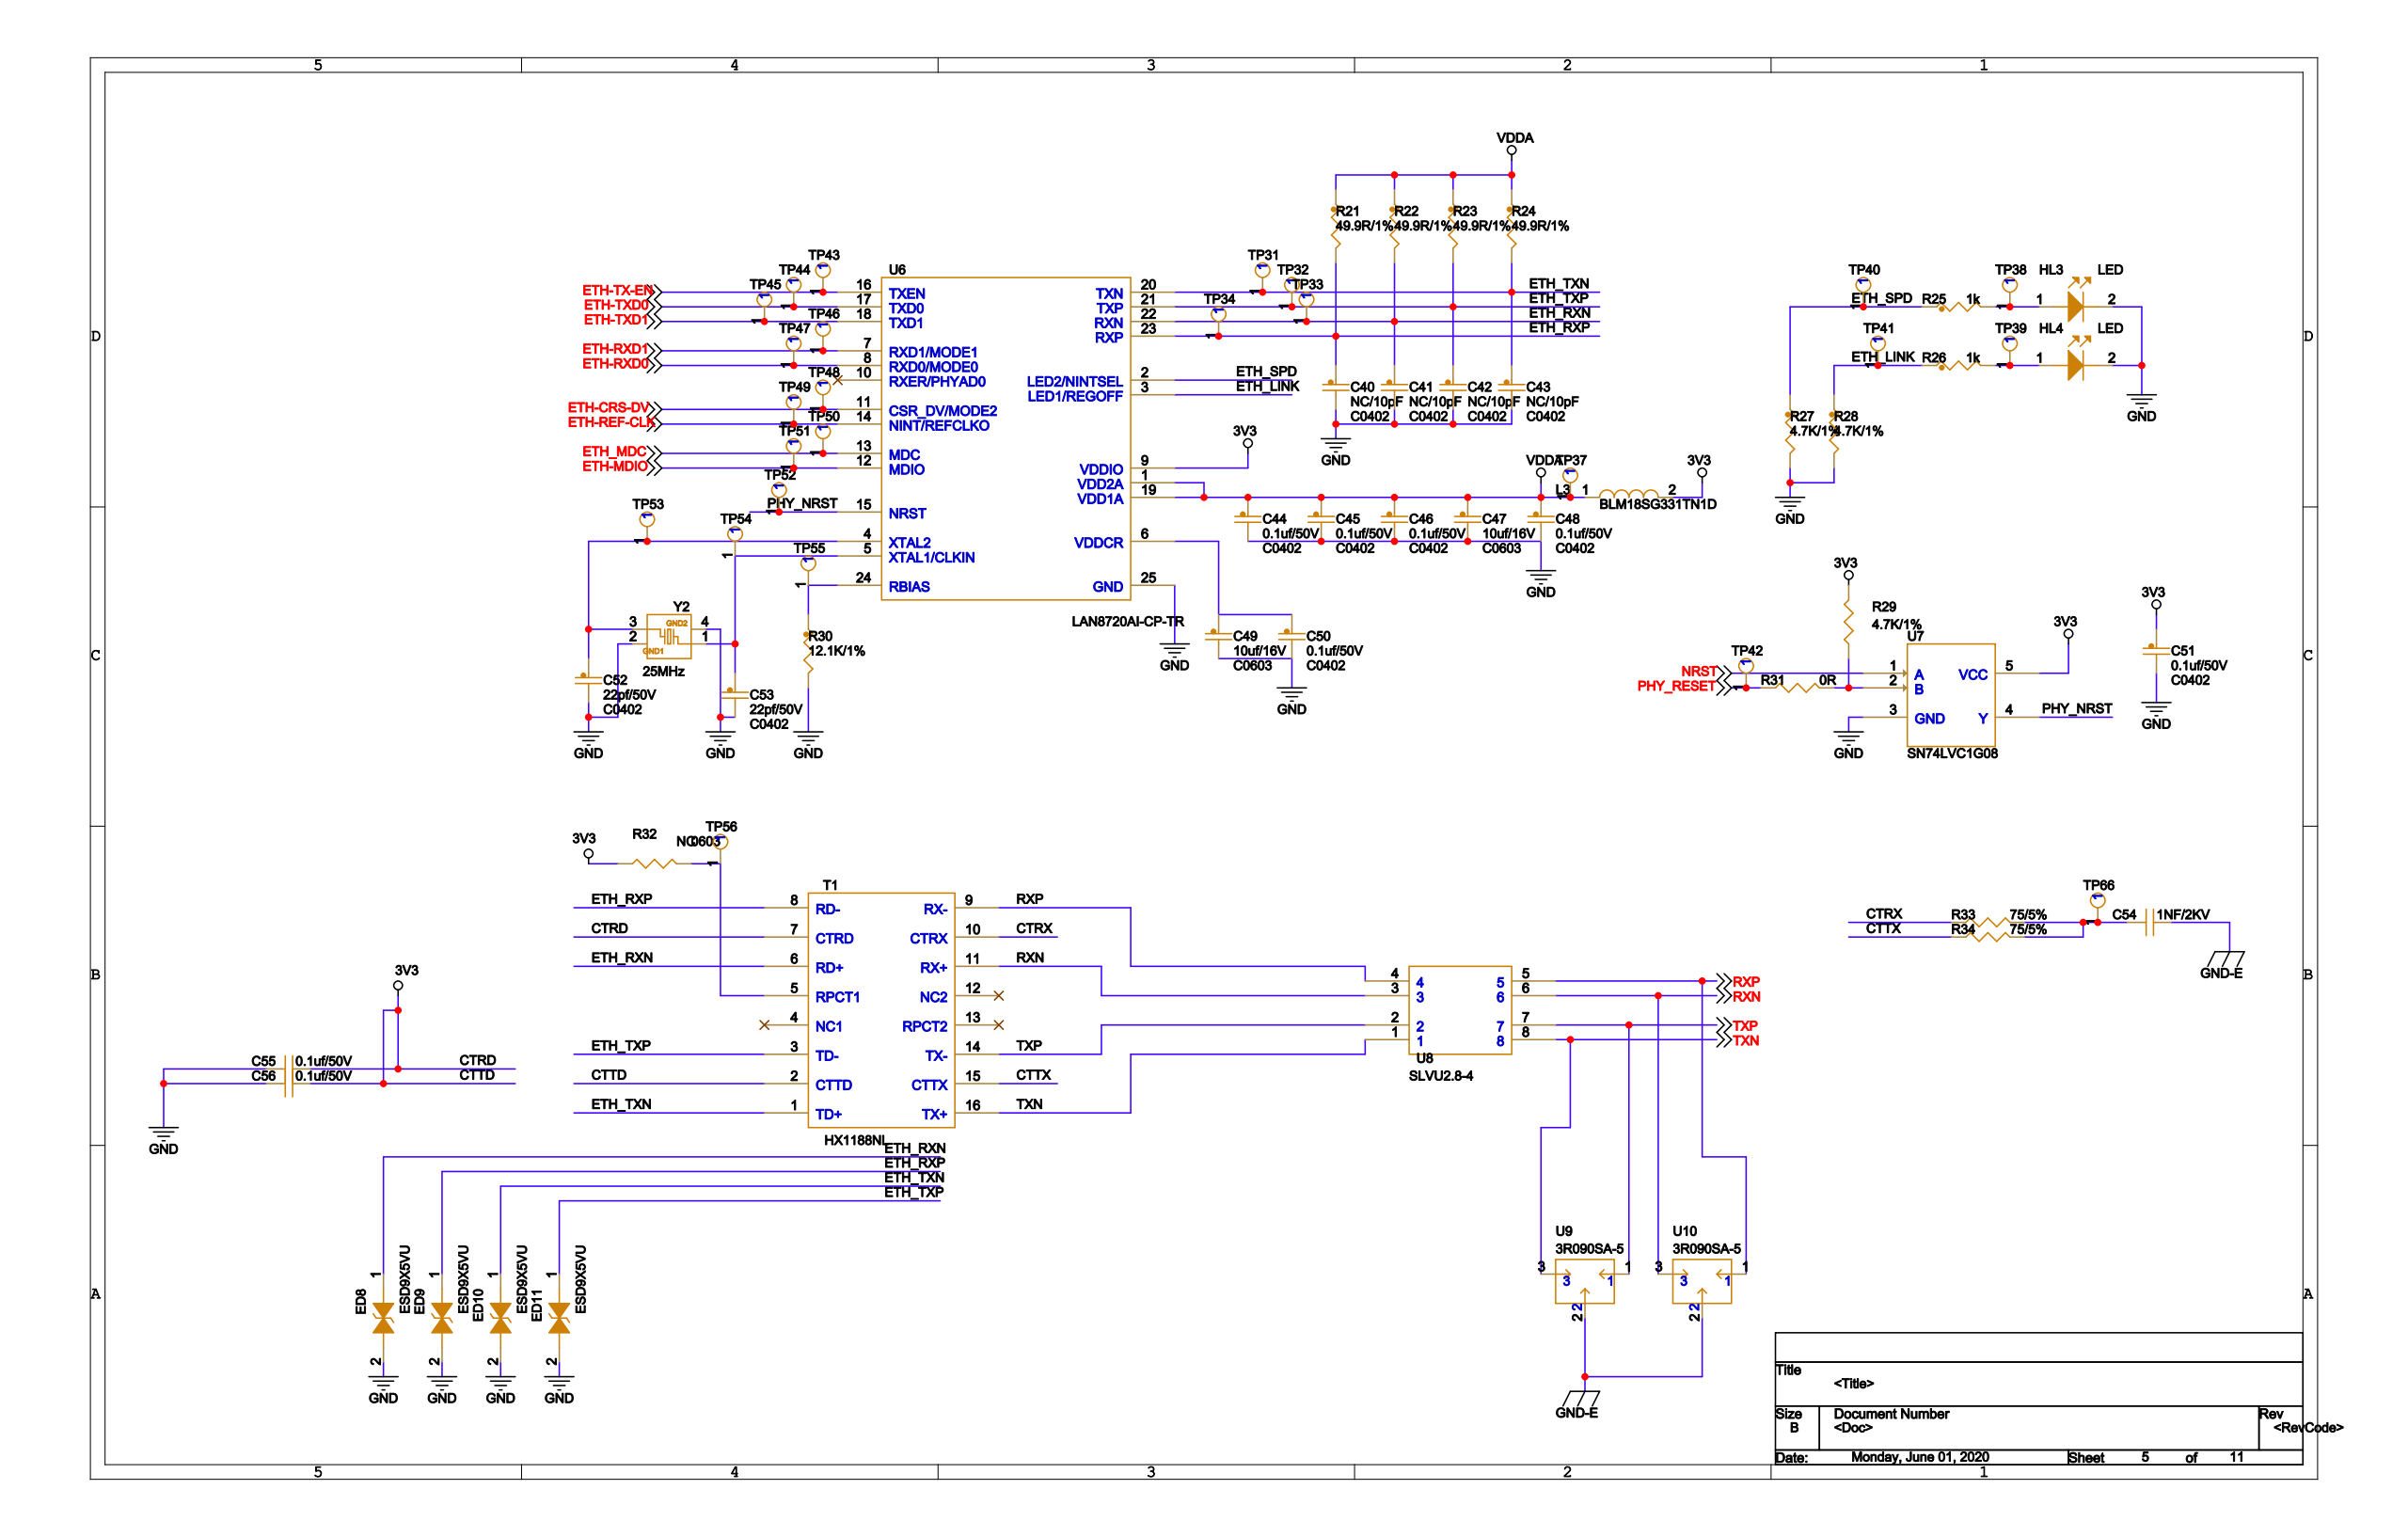Circuit board | Cadence Allegro | 792 parts | 400 nets | one sheet of the schematic
Parts on this sheet (reference | value | footprint):
C40 | NC/10pF | C0402
C41 | NC/10pF | C0402
C42 | NC/10pF | C0402
C43 | NC/10pF | C0402
C44 | 0.1uf/50V | C0402
C45 | 0.1uf/50V | C0402
C46 | 0.1uf/50V | C0402
C47 | 10uf/16V | C0603
C48 | 0.1uf/50V | C0402
C49 | 10uf/16V | C0603
C50 | 0.1uf/50V | C0402
C51 | 0.1uf/50V | C0402
C52 | 22pf/50V | C0402
C53 | 22pf/50V | C0402
C54 | 1NF/2KV | C1210
C55 | 0.1uf/50V | C0402
C56 | 0.1uf/50V | C0402
ED8 | ESD9X5VU | ESD5Z12T1
ED9 | ESD9X5VU | ESD5Z12T1
ED10 | ESD9X5VU | ESD5Z12T1
ED11 | ESD9X5VU | ESD5Z12T1
HL3 | LED | LED0603
HL4 | LED | LED0603
L3 | BLM18SG331TN1D | 0603
R21 | 49.9R/1% | 0603
R22 | 49.9R/1% | 0603
R23 | 49.9R/1% | 0603
R24 | 49.9R/1% | 0603
R25 | 1k | 0603
R26 | 1k | 0603
R27 | 4.7K/1% | 0402
R28 | 4.7K/1% | 0402
R29 | 4.7K/1% | 0402
R30 | 12.1K/1% | 0603
R31 | 0R | 0603
R32 | NC | 0603
R33 | 75/5% | 1206
R34 | 75/5% | 1206
T1 | HX1188NL | TRANS_H1102
TP31 | TESTPOINT | TESTPOINT-33MIL
TP32 | TESTPOINT | TESTPOINT-33MIL
TP33 | TESTPOINT | TESTPOINT-33MIL
TP34 | TESTPOINT | TESTPOINT-33MIL
TP37 | TESTPOINT | TESTPOINT-33MIL
TP38 | TESTPOINT | TESTPOINT-33MIL
TP39 | TESTPOINT | TESTPOINT-33MIL
TP40 | TESTPOINT | TESTPOINT-33MIL
TP41 | TESTPOINT | TESTPOINT-33MIL
TP42 | TESTPOINT | TESTPOINT-33MIL
TP43 | TESTPOINT | TESTPOINT-33MIL
TP44 | TESTPOINT | TESTPOINT-33MIL
TP45 | TESTPOINT | TESTPOINT-33MIL
TP46 | TESTPOINT | TESTPOINT-33MIL
TP47 | TESTPOINT | TESTPOINT-33MIL
TP48 | TESTPOINT | TESTPOINT-33MIL
TP49 | TESTPOINT | TESTPOINT-33MIL
TP50 | TESTPOINT | TESTPOINT-33MIL
TP52 | TESTPOINT | TESTPOINT-33MIL
TP53 | TESTPOINT | TESTPOINT-33MIL
TP54 | TESTPOINT | TESTPOINT-33MIL
TP55 | TESTPOINT | TESTPOINT-33MIL
TP56 | TESTPOINT | TESTPOINT-33MIL
TP66 | TESTPOINT | TESTPOINT-33MIL
U6 | LAN8720AI-CP-TR | QFN24
U7 | SN74LVC1G08 | SC70_5PIN
U8 | SLVU2.8-4 | SOP8
U9 | 3R090SA-5 | 3R090SA-5
U10 | 3R090SA-5 | 3R090SA-5
Y2 | 25MHz | OSC_SMD3L2X2L5
Nets of these parts (net: part-pin ...):
3V3: C51-1 C55-1 C56-1 L3-2 R29-2 R32-1 T1-2 T1-7 U7-5 U6-9
GND-E: C54-1 U9-2 U10-2
GND: C40-2 C41-2 C42-2 C43-2 C44-2 C45-2 C46-2 C47-2 C48-2 C49-2 C50-2 C51-2 C52-2 C53-2 C55-2 C56-2 ED8-2 ED9-2 ED10-2 ED11-2 HL3-2 HL4-2 R27-2 R28-2 R30-2 U7-3 Y2-2 Y2-4 U6-25
RXN: T1-11 U8-3 U8-6 U10-3
TXP: T1-14 U8-2 U8-7 U9-1
RXP: T1-9 U8-4 U8-5 U10-1
TXN: T1-16 U8-1 U8-8 U9-3
ETH_TXN: C43-1 ED10-1 R24-2 T1-1 TP31-1 U6-20
ETH_TXP: C42-1 ED11-1 R23-2 T1-3 TP32-1 U6-21
ETH_RXN: C41-1 ED8-1 R22-2 T1-6 TP33-1 U6-22
ETH_RXP: C40-1 ED9-1 R21-2 T1-8 TP34-1 U6-23
NRST: U7-1
VDDA: C44-1 C45-1 C46-1 C47-1 C48-1 L3-1 R21-1 R22-1 R23-1 R24-1 TP37-1 U6-1 U6-19
N7261762: HL3-1 R25-2 TP38-1
N7261772: HL4-1 R26-2 TP39-1
ETH_SPD: R25-1 R27-1 TP40-1 U6-2
ETH_LINK: R26-1 R28-1 TP41-1 U6-3
PHY_RESET: R31-1 TP42-1
ETH-TX-EN: TP43-1 U6-16
ETH-TXD0: TP44-1 U6-17
ETH-TXD1: TP45-1 U6-18
ETH-RXD1: TP46-1 U6-7
ETH-RXD0: TP47-1 U6-8
ETH-CRS-DV: TP48-1 U6-11
ETH-REF-CLK: TP49-1 U6-14
ETH_MDC: TP50-1 U6-13
ETH-MDIO: U6-12
PHY_NRST: TP52-1 U7-4 U6-15
N13416: C52-1 TP53-1 Y2-3 U6-4
N13448: C53-1 TP54-1 Y2-1 U6-5
N13556: R30-1 TP55-1 U6-24
N7186602: R32-2 T1-5 TP56-1
N7186980: C54-2 R33-2 R34-2 TP66-1
N7361898: R29-1 R31-2 U7-2
N15756: C49-1 C50-1 U6-6
CTRX: R33-1 T1-10
CTTX: R34-1 T1-15